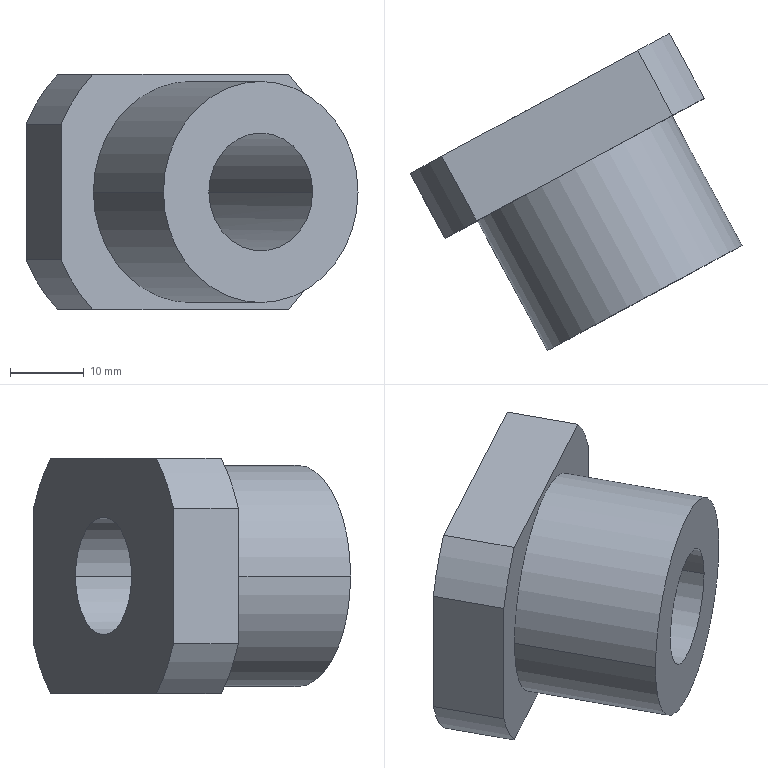Part | Creo | 1 solid | 15 faces | box 45.051 x 43.028 x 32 mm | volume 20327 mm3 | cylinder 8 | plane 7 | commonest cylinder face diameters 44 x4 16 x2 30 x2
STEP:
#1=CARTESIAN_POINT('',(0.,0.,0.));
#2=DIRECTION('',(0.,0.,1.));
#3=DIRECTION('',(1.,0.,0.));
#4=AXIS2_PLACEMENT_3D('',#1,#2,#3);
#5=CARTESIAN_POINT('',(319.736,-158.085,-84.939));
#6=VERTEX_POINT('',#5);
#7=CARTESIAN_POINT('',(315.424,-160.413,-91.774));
#8=VERTEX_POINT('',#7);
#9=CARTESIAN_POINT('',(302.138,-167.588,-75.774));
#10=DIRECTION('',(-0.4752,0.8799,0.));
#11=DIRECTION('',(0.7999,0.432,-0.4166));
#12=AXIS2_PLACEMENT_3D('',#9,#10,#11);
#13=CIRCLE('',#12,22.);
#14=EDGE_CURVE('',#6,#8,#13,.T.);
#15=ORIENTED_EDGE('',*,*,#14,.T.);
#16=CARTESIAN_POINT('',(320.175,-169.212,-91.774));
#17=VERTEX_POINT('',#16);
#18=CARTESIAN_POINT('',(315.424,-160.413,-91.774));
#19=DIRECTION('',(0.4752,-0.8799,0.));
#20=VECTOR('',#19,10.);
#21=LINE('',#18,#20);
#22=EDGE_CURVE('',#8,#17,#21,.T.);
#23=ORIENTED_EDGE('',*,*,#22,.T.);
#24=CARTESIAN_POINT('',(324.487,-166.884,-84.939));
#25=VERTEX_POINT('',#24);
#26=CARTESIAN_POINT('',(306.889,-176.387,-75.774));
#27=DIRECTION('',(0.4752,-0.8799,0.));
#28=DIRECTION('',(0.6039,0.3261,-0.7273));
#29=AXIS2_PLACEMENT_3D('',#26,#27,#28);
#30=CIRCLE('',#29,22.);
#31=EDGE_CURVE('',#17,#25,#30,.T.);
#32=ORIENTED_EDGE('',*,*,#31,.T.);
#33=CARTESIAN_POINT('',(319.736,-158.085,-84.939));
#34=DIRECTION('',(0.4752,-0.8799,0.));
#35=VECTOR('',#34,10.);
#36=LINE('',#33,#35);
#37=EDGE_CURVE('',#6,#25,#36,.T.);
#38=ORIENTED_EDGE('',*,*,#37,.F.);
#39=EDGE_LOOP('',(#15,#23,#32,#38));
#40=FACE_OUTER_BOUND('',#39,.F.);
#41=CARTESIAN_POINT('',(302.138,-167.588,-75.774));
#42=DIRECTION('',(0.4752,-0.8799,0.));
#43=DIRECTION('',(0.8799,0.4752,0.));
#44=AXIS2_PLACEMENT_3D('',#41,#42,#43);
#45=CYLINDRICAL_SURFACE('',#44,22.);
#46=ADVANCED_FACE('',(#40),#45,.T.);
#47=CARTESIAN_POINT('',(288.851,-174.763,-91.774));
#48=VERTEX_POINT('',#47);
#49=CARTESIAN_POINT('',(288.851,-174.763,-91.774));
#50=DIRECTION('',(0.8799,0.4752,0.));
#51=VECTOR('',#50,30.199);
#52=LINE('',#49,#51);
#53=EDGE_CURVE('',#48,#8,#52,.T.);
#54=ORIENTED_EDGE('',*,*,#53,.T.);
#55=ORIENTED_EDGE('',*,*,#14,.F.);
#56=CARTESIAN_POINT('',(319.736,-158.085,-66.609));
#57=VERTEX_POINT('',#56);
#58=CARTESIAN_POINT('',(319.736,-158.085,-66.609));
#59=DIRECTION('',(0.,0.,-1.));
#60=VECTOR('',#59,18.33);
#61=LINE('',#58,#60);
#62=EDGE_CURVE('',#57,#6,#61,.T.);
#63=ORIENTED_EDGE('',*,*,#62,.F.);
#64=CARTESIAN_POINT('',(315.424,-160.413,-59.774));
#65=VERTEX_POINT('',#64);
#66=CARTESIAN_POINT('',(302.138,-167.588,-75.774));
#67=DIRECTION('',(-0.4752,0.8799,0.));
#68=DIRECTION('',(0.6039,0.3261,0.7273));
#69=AXIS2_PLACEMENT_3D('',#66,#67,#68);
#70=CIRCLE('',#69,22.);
#71=EDGE_CURVE('',#65,#57,#70,.T.);
#72=ORIENTED_EDGE('',*,*,#71,.F.);
#73=CARTESIAN_POINT('',(288.851,-174.763,-59.774));
#74=VERTEX_POINT('',#73);
#75=CARTESIAN_POINT('',(315.424,-160.413,-59.774));
#76=DIRECTION('',(-0.8799,-0.4752,0.));
#77=VECTOR('',#76,30.199);
#78=LINE('',#75,#77);
#79=EDGE_CURVE('',#65,#74,#78,.T.);
#80=ORIENTED_EDGE('',*,*,#79,.T.);
#81=CARTESIAN_POINT('',(284.54,-177.091,-66.609));
#82=VERTEX_POINT('',#81);
#83=CARTESIAN_POINT('',(302.138,-167.588,-75.774));
#84=DIRECTION('',(-0.4752,0.8799,0.));
#85=DIRECTION('',(-0.7999,-0.432,0.4166));
#86=AXIS2_PLACEMENT_3D('',#83,#84,#85);
#87=CIRCLE('',#86,22.);
#88=EDGE_CURVE('',#82,#74,#87,.T.);
#89=ORIENTED_EDGE('',*,*,#88,.F.);
#90=CARTESIAN_POINT('',(284.54,-177.091,-84.939));
#91=VERTEX_POINT('',#90);
#92=CARTESIAN_POINT('',(284.54,-177.091,-66.609));
#93=DIRECTION('',(0.,0.,-1.));
#94=VECTOR('',#93,18.33);
#95=LINE('',#92,#94);
#96=EDGE_CURVE('',#82,#91,#95,.T.);
#97=ORIENTED_EDGE('',*,*,#96,.T.);
#98=CARTESIAN_POINT('',(302.138,-167.588,-75.774));
#99=DIRECTION('',(-0.4752,0.8799,0.));
#100=DIRECTION('',(-0.6039,-0.3261,-0.7273));
#101=AXIS2_PLACEMENT_3D('',#98,#99,#100);
#102=CIRCLE('',#101,22.);
#103=EDGE_CURVE('',#48,#91,#102,.T.);
#104=ORIENTED_EDGE('',*,*,#103,.F.);
#105=EDGE_LOOP('',(#54,#55,#63,#72,#80,#89,#97,#104));
#106=FACE_OUTER_BOUND('',#105,.F.);
#107=CARTESIAN_POINT('',(302.138,-167.588,-67.774));
#108=VERTEX_POINT('',#107);
#109=CARTESIAN_POINT('',(295.098,-171.389,-75.774));
#110=VERTEX_POINT('',#109);
#111=CARTESIAN_POINT('',(302.138,-167.588,-75.774));
#112=DIRECTION('',(0.4752,-0.8799,0.));
#113=DIRECTION('',(0.,0.,1.));
#114=AXIS2_PLACEMENT_3D('',#111,#112,#113);
#115=CIRCLE('',#114,8.);
#116=EDGE_CURVE('',#108,#110,#115,.T.);
#117=ORIENTED_EDGE('',*,*,#116,.F.);
#118=CARTESIAN_POINT('',(309.177,-163.787,-75.774));
#119=VERTEX_POINT('',#118);
#120=CARTESIAN_POINT('',(302.138,-167.588,-75.774));
#121=DIRECTION('',(0.4752,-0.8799,0.));
#122=DIRECTION('',(0.8799,0.4752,0.));
#123=AXIS2_PLACEMENT_3D('',#120,#121,#122);
#124=CIRCLE('',#123,8.);
#125=EDGE_CURVE('',#119,#108,#124,.T.);
#126=ORIENTED_EDGE('',*,*,#125,.F.);
#127=CARTESIAN_POINT('',(302.138,-167.588,-83.774));
#128=VERTEX_POINT('',#127);
#129=CARTESIAN_POINT('',(302.138,-167.588,-75.774));
#130=DIRECTION('',(0.4752,-0.8799,0.));
#131=DIRECTION('',(0.,0.,-1.));
#132=AXIS2_PLACEMENT_3D('',#129,#130,#131);
#133=CIRCLE('',#132,8.);
#134=EDGE_CURVE('',#128,#119,#133,.T.);
#135=ORIENTED_EDGE('',*,*,#134,.F.);
#136=CARTESIAN_POINT('',(302.138,-167.588,-75.774));
#137=DIRECTION('',(0.4752,-0.8799,0.));
#138=DIRECTION('',(-0.8799,-0.4752,0.));
#139=AXIS2_PLACEMENT_3D('',#136,#137,#138);
#140=CIRCLE('',#139,8.);
#141=EDGE_CURVE('',#110,#128,#140,.T.);
#142=ORIENTED_EDGE('',*,*,#141,.F.);
#143=EDGE_LOOP('',(#117,#126,#135,#142));
#144=FACE_BOUND('',#143,.F.);
#145=CARTESIAN_POINT('',(302.138,-167.588,-75.774));
#146=DIRECTION('',(-0.4752,0.8799,0.));
#147=DIRECTION('',(-0.8799,-0.4752,0.));
#148=AXIS2_PLACEMENT_3D('',#145,#146,#147);
#149=PLANE('',#148);
#150=ADVANCED_FACE('',(#106,#144),#149,.T.);
#151=ORIENTED_EDGE('',*,*,#53,.F.);
#152=CARTESIAN_POINT('',(293.603,-183.562,-91.774));
#153=VERTEX_POINT('',#152);
#154=CARTESIAN_POINT('',(293.603,-183.562,-91.774));
#155=DIRECTION('',(-0.4752,0.8799,0.));
#156=VECTOR('',#155,10.);
#157=LINE('',#154,#156);
#158=EDGE_CURVE('',#153,#48,#157,.T.);
#159=ORIENTED_EDGE('',*,*,#158,.F.);
#160=CARTESIAN_POINT('',(320.175,-169.212,-91.774));
#161=DIRECTION('',(-0.8799,-0.4752,0.));
#162=VECTOR('',#161,30.199);
#163=LINE('',#160,#162);
#164=EDGE_CURVE('',#17,#153,#163,.T.);
#165=ORIENTED_EDGE('',*,*,#164,.F.);
#166=ORIENTED_EDGE('',*,*,#22,.F.);
#167=EDGE_LOOP('',(#151,#159,#165,#166));
#168=FACE_OUTER_BOUND('',#167,.F.);
#169=CARTESIAN_POINT('',(306.889,-176.387,-91.774));
#170=DIRECTION('',(0.,0.,1.));
#171=DIRECTION('',(1.,0.,0.));
#172=AXIS2_PLACEMENT_3D('',#169,#170,#171);
#173=PLANE('',#172);
#174=ADVANCED_FACE('',(#168),#173,.F.);
#175=CARTESIAN_POINT('',(289.291,-185.89,-84.939));
#176=VERTEX_POINT('',#175);
#177=CARTESIAN_POINT('',(306.889,-176.387,-75.774));
#178=DIRECTION('',(0.4752,-0.8799,0.));
#179=DIRECTION('',(-0.7999,-0.432,-0.4166));
#180=AXIS2_PLACEMENT_3D('',#177,#178,#179);
#181=CIRCLE('',#180,22.);
#182=EDGE_CURVE('',#176,#153,#181,.T.);
#183=ORIENTED_EDGE('',*,*,#182,.T.);
#184=ORIENTED_EDGE('',*,*,#158,.T.);
#185=ORIENTED_EDGE('',*,*,#103,.T.);
#186=CARTESIAN_POINT('',(289.291,-185.89,-84.939));
#187=DIRECTION('',(-0.4752,0.8799,0.));
#188=VECTOR('',#187,10.);
#189=LINE('',#186,#188);
#190=EDGE_CURVE('',#176,#91,#189,.T.);
#191=ORIENTED_EDGE('',*,*,#190,.F.);
#192=EDGE_LOOP('',(#183,#184,#185,#191));
#193=FACE_OUTER_BOUND('',#192,.F.);
#194=CARTESIAN_POINT('',(302.138,-167.588,-75.774));
#195=DIRECTION('',(0.4752,-0.8799,0.));
#196=DIRECTION('',(0.8799,0.4752,0.));
#197=AXIS2_PLACEMENT_3D('',#194,#195,#196);
#198=CYLINDRICAL_SURFACE('',#197,22.);
#199=ADVANCED_FACE('',(#193),#198,.T.);
#200=ORIENTED_EDGE('',*,*,#164,.T.);
#201=ORIENTED_EDGE('',*,*,#182,.F.);
#202=CARTESIAN_POINT('',(289.291,-185.89,-66.609));
#203=VERTEX_POINT('',#202);
#204=CARTESIAN_POINT('',(289.291,-185.89,-84.939));
#205=DIRECTION('',(0.,0.,1.));
#206=VECTOR('',#205,18.33);
#207=LINE('',#204,#206);
#208=EDGE_CURVE('',#176,#203,#207,.T.);
#209=ORIENTED_EDGE('',*,*,#208,.T.);
#210=CARTESIAN_POINT('',(293.603,-183.562,-59.774));
#211=VERTEX_POINT('',#210);
#212=CARTESIAN_POINT('',(306.889,-176.387,-75.774));
#213=DIRECTION('',(0.4752,-0.8799,0.));
#214=DIRECTION('',(-0.6039,-0.3261,0.7273));
#215=AXIS2_PLACEMENT_3D('',#212,#213,#214);
#216=CIRCLE('',#215,22.);
#217=EDGE_CURVE('',#211,#203,#216,.T.);
#218=ORIENTED_EDGE('',*,*,#217,.F.);
#219=CARTESIAN_POINT('',(320.175,-169.212,-59.774));
#220=VERTEX_POINT('',#219);
#221=CARTESIAN_POINT('',(293.603,-183.562,-59.774));
#222=DIRECTION('',(0.8799,0.4752,0.));
#223=VECTOR('',#222,30.199);
#224=LINE('',#221,#223);
#225=EDGE_CURVE('',#211,#220,#224,.T.);
#226=ORIENTED_EDGE('',*,*,#225,.T.);
#227=CARTESIAN_POINT('',(324.487,-166.884,-66.609));
#228=VERTEX_POINT('',#227);
#229=CARTESIAN_POINT('',(306.889,-176.387,-75.774));
#230=DIRECTION('',(0.4752,-0.8799,0.));
#231=DIRECTION('',(0.7999,0.432,0.4166));
#232=AXIS2_PLACEMENT_3D('',#229,#230,#231);
#233=CIRCLE('',#232,22.);
#234=EDGE_CURVE('',#228,#220,#233,.T.);
#235=ORIENTED_EDGE('',*,*,#234,.F.);
#236=CARTESIAN_POINT('',(324.487,-166.884,-84.939));
#237=DIRECTION('',(0.,0.,1.));
#238=VECTOR('',#237,18.33);
#239=LINE('',#236,#238);
#240=EDGE_CURVE('',#25,#228,#239,.T.);
#241=ORIENTED_EDGE('',*,*,#240,.F.);
#242=ORIENTED_EDGE('',*,*,#31,.F.);
#243=EDGE_LOOP('',(#200,#201,#209,#218,#226,#235,#241,#242));
#244=FACE_OUTER_BOUND('',#243,.F.);
#245=CARTESIAN_POINT('',(306.889,-176.387,-90.774));
#246=VERTEX_POINT('',#245);
#247=CARTESIAN_POINT('',(293.691,-183.515,-75.774));
#248=VERTEX_POINT('',#247);
#249=CARTESIAN_POINT('',(306.889,-176.387,-75.774));
#250=DIRECTION('',(-0.4752,0.8799,0.));
#251=DIRECTION('',(0.,0.,-1.));
#252=AXIS2_PLACEMENT_3D('',#249,#250,#251);
#253=CIRCLE('',#252,15.);
#254=EDGE_CURVE('',#246,#248,#253,.T.);
#255=ORIENTED_EDGE('',*,*,#254,.F.);
#256=CARTESIAN_POINT('',(320.088,-169.26,-75.774));
#257=VERTEX_POINT('',#256);
#258=CARTESIAN_POINT('',(306.889,-176.387,-75.774));
#259=DIRECTION('',(-0.4752,0.8799,0.));
#260=DIRECTION('',(0.8799,0.4752,0.));
#261=AXIS2_PLACEMENT_3D('',#258,#259,#260);
#262=CIRCLE('',#261,15.);
#263=EDGE_CURVE('',#257,#246,#262,.T.);
#264=ORIENTED_EDGE('',*,*,#263,.F.);
#265=CARTESIAN_POINT('',(306.889,-176.387,-60.774));
#266=VERTEX_POINT('',#265);
#267=CARTESIAN_POINT('',(306.889,-176.387,-75.774));
#268=DIRECTION('',(-0.4752,0.8799,0.));
#269=DIRECTION('',(0.,0.,1.));
#270=AXIS2_PLACEMENT_3D('',#267,#268,#269);
#271=CIRCLE('',#270,15.);
#272=EDGE_CURVE('',#266,#257,#271,.T.);
#273=ORIENTED_EDGE('',*,*,#272,.F.);
#274=CARTESIAN_POINT('',(306.889,-176.387,-75.774));
#275=DIRECTION('',(-0.4752,0.8799,0.));
#276=DIRECTION('',(-0.8799,-0.4752,0.));
#277=AXIS2_PLACEMENT_3D('',#274,#275,#276);
#278=CIRCLE('',#277,15.);
#279=EDGE_CURVE('',#248,#266,#278,.T.);
#280=ORIENTED_EDGE('',*,*,#279,.F.);
#281=EDGE_LOOP('',(#255,#264,#273,#280));
#282=FACE_BOUND('',#281,.F.);
#283=CARTESIAN_POINT('',(306.889,-176.387,-75.774));
#284=DIRECTION('',(0.4752,-0.8799,0.));
#285=DIRECTION('',(0.8799,0.4752,0.));
#286=AXIS2_PLACEMENT_3D('',#283,#284,#285);
#287=PLANE('',#286);
#288=ADVANCED_FACE('',(#244,#282),#287,.T.);
#289=ORIENTED_EDGE('',*,*,#96,.F.);
#290=CARTESIAN_POINT('',(284.54,-177.091,-66.609));
#291=DIRECTION('',(0.4752,-0.8799,0.));
#292=VECTOR('',#291,10.);
#293=LINE('',#290,#292);
#294=EDGE_CURVE('',#82,#203,#293,.T.);
#295=ORIENTED_EDGE('',*,*,#294,.T.);
#296=ORIENTED_EDGE('',*,*,#208,.F.);
#297=ORIENTED_EDGE('',*,*,#190,.T.);
#298=EDGE_LOOP('',(#289,#295,#296,#297));
#299=FACE_OUTER_BOUND('',#298,.F.);
#300=CARTESIAN_POINT('',(289.291,-185.89,-75.774));
#301=DIRECTION('',(0.8799,0.4752,0.));
#302=DIRECTION('',(-0.4752,0.8799,0.));
#303=AXIS2_PLACEMENT_3D('',#300,#301,#302);
#304=PLANE('',#303);
#305=ADVANCED_FACE('',(#299),#304,.F.);
#306=CARTESIAN_POINT('',(288.851,-174.763,-59.774));
#307=DIRECTION('',(0.4752,-0.8799,0.));
#308=VECTOR('',#307,10.);
#309=LINE('',#306,#308);
#310=EDGE_CURVE('',#74,#211,#309,.T.);
#311=ORIENTED_EDGE('',*,*,#310,.T.);
#312=ORIENTED_EDGE('',*,*,#217,.T.);
#313=ORIENTED_EDGE('',*,*,#294,.F.);
#314=ORIENTED_EDGE('',*,*,#88,.T.);
#315=EDGE_LOOP('',(#311,#312,#313,#314));
#316=FACE_OUTER_BOUND('',#315,.F.);
#317=CARTESIAN_POINT('',(302.138,-167.588,-75.774));
#318=DIRECTION('',(0.4752,-0.8799,0.));
#319=DIRECTION('',(0.8799,0.4752,0.));
#320=AXIS2_PLACEMENT_3D('',#317,#318,#319);
#321=CYLINDRICAL_SURFACE('',#320,22.);
#322=ADVANCED_FACE('',(#316),#321,.T.);
#323=ORIENTED_EDGE('',*,*,#79,.F.);
#324=CARTESIAN_POINT('',(320.175,-169.212,-59.774));
#325=DIRECTION('',(-0.4752,0.8799,0.));
#326=VECTOR('',#325,10.);
#327=LINE('',#324,#326);
#328=EDGE_CURVE('',#220,#65,#327,.T.);
#329=ORIENTED_EDGE('',*,*,#328,.F.);
#330=ORIENTED_EDGE('',*,*,#225,.F.);
#331=ORIENTED_EDGE('',*,*,#310,.F.);
#332=EDGE_LOOP('',(#323,#329,#330,#331));
#333=FACE_OUTER_BOUND('',#332,.F.);
#334=CARTESIAN_POINT('',(306.889,-176.387,-59.774));
#335=DIRECTION('',(0.,0.,1.));
#336=DIRECTION('',(1.,0.,0.));
#337=AXIS2_PLACEMENT_3D('',#334,#335,#336);
#338=PLANE('',#337);
#339=ADVANCED_FACE('',(#333),#338,.T.);
#340=ORIENTED_EDGE('',*,*,#328,.T.);
#341=ORIENTED_EDGE('',*,*,#71,.T.);
#342=CARTESIAN_POINT('',(324.487,-166.884,-66.609));
#343=DIRECTION('',(-0.4752,0.8799,0.));
#344=VECTOR('',#343,10.);
#345=LINE('',#342,#344);
#346=EDGE_CURVE('',#228,#57,#345,.T.);
#347=ORIENTED_EDGE('',*,*,#346,.F.);
#348=ORIENTED_EDGE('',*,*,#234,.T.);
#349=EDGE_LOOP('',(#340,#341,#347,#348));
#350=FACE_OUTER_BOUND('',#349,.F.);
#351=CARTESIAN_POINT('',(302.138,-167.588,-75.774));
#352=DIRECTION('',(0.4752,-0.8799,0.));
#353=DIRECTION('',(0.8799,0.4752,0.));
#354=AXIS2_PLACEMENT_3D('',#351,#352,#353);
#355=CYLINDRICAL_SURFACE('',#354,22.);
#356=ADVANCED_FACE('',(#350),#355,.T.);
#357=ORIENTED_EDGE('',*,*,#62,.T.);
#358=ORIENTED_EDGE('',*,*,#37,.T.);
#359=ORIENTED_EDGE('',*,*,#240,.T.);
#360=ORIENTED_EDGE('',*,*,#346,.T.);
#361=EDGE_LOOP('',(#357,#358,#359,#360));
#362=FACE_OUTER_BOUND('',#361,.F.);
#363=CARTESIAN_POINT('',(324.487,-166.884,-75.774));
#364=DIRECTION('',(0.8799,0.4752,0.));
#365=DIRECTION('',(-0.4752,0.8799,0.));
#366=AXIS2_PLACEMENT_3D('',#363,#364,#365);
#367=PLANE('',#366);
#368=ADVANCED_FACE('',(#362),#367,.T.);
#369=ORIENTED_EDGE('',*,*,#263,.T.);
#370=ORIENTED_EDGE('',*,*,#254,.T.);
#371=CARTESIAN_POINT('',(303.194,-201.112,-75.774));
#372=VERTEX_POINT('',#371);
#373=CARTESIAN_POINT('',(293.691,-183.515,-75.774));
#374=DIRECTION('',(0.4752,-0.8799,0.));
#375=VECTOR('',#374,20.);
#376=LINE('',#373,#375);
#377=EDGE_CURVE('',#248,#372,#376,.T.);
#378=ORIENTED_EDGE('',*,*,#377,.T.);
#379=CARTESIAN_POINT('',(316.392,-193.985,-90.774));
#380=VERTEX_POINT('',#379);
#381=CARTESIAN_POINT('',(316.392,-193.985,-75.774));
#382=DIRECTION('',(0.4752,-0.8799,0.));
#383=DIRECTION('',(-0.8799,-0.4752,0.));
#384=AXIS2_PLACEMENT_3D('',#381,#382,#383);
#385=CIRCLE('',#384,15.);
#386=EDGE_CURVE('',#372,#380,#385,.T.);
#387=ORIENTED_EDGE('',*,*,#386,.T.);
#388=CARTESIAN_POINT('',(329.591,-186.858,-75.774));
#389=VERTEX_POINT('',#388);
#390=CARTESIAN_POINT('',(316.392,-193.985,-75.774));
#391=DIRECTION('',(0.4752,-0.8799,0.));
#392=DIRECTION('',(0.,0.,-1.));
#393=AXIS2_PLACEMENT_3D('',#390,#391,#392);
#394=CIRCLE('',#393,15.);
#395=EDGE_CURVE('',#380,#389,#394,.T.);
#396=ORIENTED_EDGE('',*,*,#395,.T.);
#397=CARTESIAN_POINT('',(320.088,-169.26,-75.774));
#398=DIRECTION('',(0.4752,-0.8799,0.));
#399=VECTOR('',#398,20.);
#400=LINE('',#397,#399);
#401=EDGE_CURVE('',#257,#389,#400,.T.);
#402=ORIENTED_EDGE('',*,*,#401,.F.);
#403=EDGE_LOOP('',(#369,#370,#378,#387,#396,#402));
#404=FACE_OUTER_BOUND('',#403,.F.);
#405=CARTESIAN_POINT('',(302.138,-167.588,-75.774));
#406=DIRECTION('',(0.4752,-0.8799,0.));
#407=DIRECTION('',(0.8799,0.4752,0.));
#408=AXIS2_PLACEMENT_3D('',#405,#406,#407);
#409=CYLINDRICAL_SURFACE('',#408,15.);
#410=ADVANCED_FACE('',(#404),#409,.T.);
#411=ORIENTED_EDGE('',*,*,#272,.T.);
#412=ORIENTED_EDGE('',*,*,#401,.T.);
#413=CARTESIAN_POINT('',(316.392,-193.985,-60.774));
#414=VERTEX_POINT('',#413);
#415=CARTESIAN_POINT('',(316.392,-193.985,-75.774));
#416=DIRECTION('',(0.4752,-0.8799,0.));
#417=DIRECTION('',(0.8799,0.4752,0.));
#418=AXIS2_PLACEMENT_3D('',#415,#416,#417);
#419=CIRCLE('',#418,15.);
#420=EDGE_CURVE('',#389,#414,#419,.T.);
#421=ORIENTED_EDGE('',*,*,#420,.T.);
#422=CARTESIAN_POINT('',(316.392,-193.985,-75.774));
#423=DIRECTION('',(0.4752,-0.8799,0.));
#424=DIRECTION('',(0.,0.,1.));
#425=AXIS2_PLACEMENT_3D('',#422,#423,#424);
#426=CIRCLE('',#425,15.);
#427=EDGE_CURVE('',#414,#372,#426,.T.);
#428=ORIENTED_EDGE('',*,*,#427,.T.);
#429=ORIENTED_EDGE('',*,*,#377,.F.);
#430=ORIENTED_EDGE('',*,*,#279,.T.);
#431=EDGE_LOOP('',(#411,#412,#421,#428,#429,#430));
#432=FACE_OUTER_BOUND('',#431,.F.);
#433=CARTESIAN_POINT('',(302.138,-167.588,-75.774));
#434=DIRECTION('',(0.4752,-0.8799,0.));
#435=DIRECTION('',(0.8799,0.4752,0.));
#436=AXIS2_PLACEMENT_3D('',#433,#434,#435);
#437=CYLINDRICAL_SURFACE('',#436,15.);
#438=ADVANCED_FACE('',(#432),#437,.T.);
#439=ORIENTED_EDGE('',*,*,#427,.F.);
#440=ORIENTED_EDGE('',*,*,#420,.F.);
#441=ORIENTED_EDGE('',*,*,#395,.F.);
#442=ORIENTED_EDGE('',*,*,#386,.F.);
#443=EDGE_LOOP('',(#439,#440,#441,#442));
#444=FACE_OUTER_BOUND('',#443,.F.);
#445=CARTESIAN_POINT('',(316.392,-193.985,-67.774));
#446=VERTEX_POINT('',#445);
#447=CARTESIAN_POINT('',(323.432,-190.184,-75.774));
#448=VERTEX_POINT('',#447);
#449=CARTESIAN_POINT('',(316.392,-193.985,-75.774));
#450=DIRECTION('',(-0.4752,0.8799,0.));
#451=DIRECTION('',(0.,0.,1.));
#452=AXIS2_PLACEMENT_3D('',#449,#450,#451);
#453=CIRCLE('',#452,8.);
#454=EDGE_CURVE('',#446,#448,#453,.T.);
#455=ORIENTED_EDGE('',*,*,#454,.F.);
#456=CARTESIAN_POINT('',(309.353,-197.786,-75.774));
#457=VERTEX_POINT('',#456);
#458=CARTESIAN_POINT('',(316.392,-193.985,-75.774));
#459=DIRECTION('',(-0.4752,0.8799,0.));
#460=DIRECTION('',(-0.8799,-0.4752,0.));
#461=AXIS2_PLACEMENT_3D('',#458,#459,#460);
#462=CIRCLE('',#461,8.);
#463=EDGE_CURVE('',#457,#446,#462,.T.);
#464=ORIENTED_EDGE('',*,*,#463,.F.);
#465=CARTESIAN_POINT('',(316.392,-193.985,-75.774));
#466=DIRECTION('',(-0.4752,0.8799,0.));
#467=DIRECTION('',(0.8799,0.4752,0.));
#468=AXIS2_PLACEMENT_3D('',#465,#466,#467);
#469=CIRCLE('',#468,8.);
#470=EDGE_CURVE('',#448,#457,#469,.T.);
#471=ORIENTED_EDGE('',*,*,#470,.F.);
#472=EDGE_LOOP('',(#455,#464,#471));
#473=FACE_BOUND('',#472,.F.);
#474=CARTESIAN_POINT('',(316.392,-193.985,-75.774));
#475=DIRECTION('',(-0.4752,0.8799,0.));
#476=DIRECTION('',(-0.8799,-0.4752,0.));
#477=AXIS2_PLACEMENT_3D('',#474,#475,#476);
#478=PLANE('',#477);
#479=ADVANCED_FACE('',(#444,#473),#478,.F.);
#480=ORIENTED_EDGE('',*,*,#125,.T.);
#481=ORIENTED_EDGE('',*,*,#116,.T.);
#482=CARTESIAN_POINT('',(295.098,-171.389,-75.774));
#483=DIRECTION('',(0.4752,-0.8799,0.));
#484=VECTOR('',#483,30.);
#485=LINE('',#482,#484);
#486=EDGE_CURVE('',#110,#457,#485,.T.);
#487=ORIENTED_EDGE('',*,*,#486,.T.);
#488=ORIENTED_EDGE('',*,*,#463,.T.);
#489=ORIENTED_EDGE('',*,*,#454,.T.);
#490=CARTESIAN_POINT('',(309.177,-163.787,-75.774));
#491=DIRECTION('',(0.4752,-0.8799,0.));
#492=VECTOR('',#491,30.);
#493=LINE('',#490,#492);
#494=EDGE_CURVE('',#119,#448,#493,.T.);
#495=ORIENTED_EDGE('',*,*,#494,.F.);
#496=EDGE_LOOP('',(#480,#481,#487,#488,#489,#495));
#497=FACE_OUTER_BOUND('',#496,.F.);
#498=CARTESIAN_POINT('',(302.138,-167.588,-75.774));
#499=DIRECTION('',(0.4752,-0.8799,0.));
#500=DIRECTION('',(0.8799,0.4752,0.));
#501=AXIS2_PLACEMENT_3D('',#498,#499,#500);
#502=CYLINDRICAL_SURFACE('',#501,8.);
#503=ADVANCED_FACE('',(#497),#502,.F.);
#504=ORIENTED_EDGE('',*,*,#134,.T.);
#505=ORIENTED_EDGE('',*,*,#494,.T.);
#506=ORIENTED_EDGE('',*,*,#470,.T.);
#507=ORIENTED_EDGE('',*,*,#486,.F.);
#508=ORIENTED_EDGE('',*,*,#141,.T.);
#509=EDGE_LOOP('',(#504,#505,#506,#507,#508));
#510=FACE_OUTER_BOUND('',#509,.F.);
#511=CARTESIAN_POINT('',(302.138,-167.588,-75.774));
#512=DIRECTION('',(0.4752,-0.8799,0.));
#513=DIRECTION('',(0.8799,0.4752,0.));
#514=AXIS2_PLACEMENT_3D('',#511,#512,#513);
#515=CYLINDRICAL_SURFACE('',#514,8.);
#516=ADVANCED_FACE('',(#510),#515,.F.);
#517=CLOSED_SHELL('',(#46,#150,#174,#199,#288,#305,#322,#339,#356,#368,#410,#438,#479,#503,#516));
#518=MANIFOLD_SOLID_BREP('',#517);
#519=(LENGTH_UNIT()NAMED_UNIT(*)SI_UNIT(.MILLI.,.METRE.));
#520=UNCERTAINTY_MEASURE_WITH_UNIT(LENGTH_MEASURE(0.007003),#519,'','');
#521=(NAMED_UNIT(*)PLANE_ANGLE_UNIT()SI_UNIT($,.RADIAN.));
#522=PLANE_ANGLE_MEASURE_WITH_UNIT(PLANE_ANGLE_MEASURE(0.01745),#521);
#523=(CONVERSION_BASED_UNIT('DEGREE',#522)NAMED_UNIT(*)PLANE_ANGLE_UNIT());
#524=(NAMED_UNIT(*)SI_UNIT($,.STERADIAN.)SOLID_ANGLE_UNIT());
#525=(GEOMETRIC_REPRESENTATION_CONTEXT(3)GLOBAL_UNCERTAINTY_ASSIGNED_CONTEXT((#520))GLOBAL_UNIT_ASSIGNED_CONTEXT((#519,#523,#524))REPRESENTATION_CONTEXT('',''));
#526=ADVANCED_BREP_SHAPE_REPRESENTATION('',(#4,#518),#525);